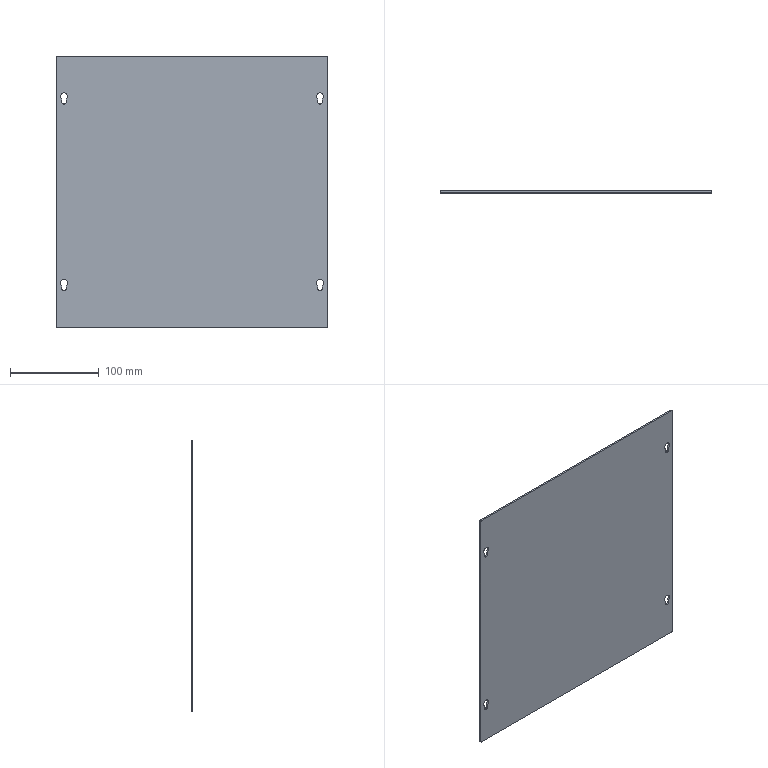Part | SolidWorks | features Fillet 1, FlatPattern 1, ICE 1, LPattern 1, SMBaseFlange 1, SheetMetal 1 | 1 solid | 30 faces | box 304.8 x 2 x 304.8 mm | volume 185210 mm3 | cylinder 16 | plane 14 | commonest cylinder face diameters 8 x8 2 x4 5.4 x4
STEP:
#1=CARTESIAN_POINT('',(-144.,-2.,111.6));
#2=VERTEX_POINT('',#1);
#3=CARTESIAN_POINT('',(-141.3,-2.,104.649));
#4=VERTEX_POINT('',#3);
#5=CARTESIAN_POINT('',(-144.,-2.,107.6));
#6=DIRECTION('',(0.,1.,0.));
#7=DIRECTION('',(0.,0.,1.));
#8=AXIS2_PLACEMENT_3D('',#5,#6,#7);
#9=CIRCLE('',#8,4.);
#10=EDGE_CURVE('',#2,#4,#9,.T.);
#11=ORIENTED_EDGE('',*,*,#10,.F.);
#12=CARTESIAN_POINT('',(-144.,0.,111.6));
#13=VERTEX_POINT('',#12);
#14=CARTESIAN_POINT('',(-144.,-10.,111.6));
#15=DIRECTION('',(0.,1.,0.));
#16=VECTOR('',#15,1000.);
#17=LINE('',#14,#16);
#18=EDGE_CURVE('',#2,#13,#17,.T.);
#19=ORIENTED_EDGE('',*,*,#18,.T.);
#20=CARTESIAN_POINT('',(-141.3,0.,104.649));
#21=VERTEX_POINT('',#20);
#22=CARTESIAN_POINT('',(-144.,0.,107.6));
#23=DIRECTION('',(0.,1.,0.));
#24=DIRECTION('',(0.,0.,1.));
#25=AXIS2_PLACEMENT_3D('',#22,#23,#24);
#26=CIRCLE('',#25,4.);
#27=EDGE_CURVE('',#13,#21,#26,.T.);
#28=ORIENTED_EDGE('',*,*,#27,.T.);
#29=CARTESIAN_POINT('',(-141.3,-10.,104.649));
#30=DIRECTION('',(0.,1.,0.));
#31=VECTOR('',#30,1000.);
#32=LINE('',#29,#31);
#33=EDGE_CURVE('',#4,#21,#32,.T.);
#34=ORIENTED_EDGE('',*,*,#33,.F.);
#35=EDGE_LOOP('',(#11,#19,#28,#34));
#36=FACE_OUTER_BOUND('',#35,.T.);
#37=CARTESIAN_POINT('',(-144.,-10.,107.6));
#38=DIRECTION('',(0.,1.,0.));
#39=DIRECTION('',(0.,0.,1.));
#40=AXIS2_PLACEMENT_3D('',#37,#38,#39);
#41=CYLINDRICAL_SURFACE('',#40,4.);
#42=ADVANCED_FACE('',(#36),#41,.F.);
#43=CARTESIAN_POINT('',(144.,-2.,111.6));
#44=VERTEX_POINT('',#43);
#45=CARTESIAN_POINT('',(146.7,-2.,104.649));
#46=VERTEX_POINT('',#45);
#47=CARTESIAN_POINT('',(144.,-2.,107.6));
#48=DIRECTION('',(0.,1.,0.));
#49=DIRECTION('',(0.,0.,1.));
#50=AXIS2_PLACEMENT_3D('',#47,#48,#49);
#51=CIRCLE('',#50,4.);
#52=EDGE_CURVE('',#44,#46,#51,.T.);
#53=ORIENTED_EDGE('',*,*,#52,.F.);
#54=CARTESIAN_POINT('',(144.,0.,111.6));
#55=VERTEX_POINT('',#54);
#56=CARTESIAN_POINT('',(144.,-10.,111.6));
#57=DIRECTION('',(0.,1.,0.));
#58=VECTOR('',#57,1000.);
#59=LINE('',#56,#58);
#60=EDGE_CURVE('',#44,#55,#59,.T.);
#61=ORIENTED_EDGE('',*,*,#60,.T.);
#62=CARTESIAN_POINT('',(146.7,0.,104.649));
#63=VERTEX_POINT('',#62);
#64=CARTESIAN_POINT('',(144.,0.,107.6));
#65=DIRECTION('',(0.,1.,0.));
#66=DIRECTION('',(0.,0.,-1.));
#67=AXIS2_PLACEMENT_3D('',#64,#65,#66);
#68=CIRCLE('',#67,4.);
#69=EDGE_CURVE('',#55,#63,#68,.T.);
#70=ORIENTED_EDGE('',*,*,#69,.T.);
#71=CARTESIAN_POINT('',(146.7,-10.,104.649));
#72=DIRECTION('',(0.,1.,0.));
#73=VECTOR('',#72,1000.);
#74=LINE('',#71,#73);
#75=EDGE_CURVE('',#46,#63,#74,.T.);
#76=ORIENTED_EDGE('',*,*,#75,.F.);
#77=EDGE_LOOP('',(#53,#61,#70,#76));
#78=FACE_OUTER_BOUND('',#77,.T.);
#79=CARTESIAN_POINT('',(144.,-10.,107.6));
#80=DIRECTION('',(0.,1.,0.));
#81=DIRECTION('',(0.,0.,1.));
#82=AXIS2_PLACEMENT_3D('',#79,#80,#81);
#83=CYLINDRICAL_SURFACE('',#82,4.);
#84=ADVANCED_FACE('',(#78),#83,.F.);
#85=CARTESIAN_POINT('',(-144.,-2.,-98.4));
#86=VERTEX_POINT('',#85);
#87=CARTESIAN_POINT('',(-141.3,-2.,-105.351));
#88=VERTEX_POINT('',#87);
#89=CARTESIAN_POINT('',(-144.,-2.,-102.4));
#90=DIRECTION('',(0.,1.,0.));
#91=DIRECTION('',(0.,0.,1.));
#92=AXIS2_PLACEMENT_3D('',#89,#90,#91);
#93=CIRCLE('',#92,4.);
#94=EDGE_CURVE('',#86,#88,#93,.T.);
#95=ORIENTED_EDGE('',*,*,#94,.F.);
#96=CARTESIAN_POINT('',(-144.,0.,-98.4));
#97=VERTEX_POINT('',#96);
#98=CARTESIAN_POINT('',(-144.,-10.,-98.4));
#99=DIRECTION('',(0.,1.,0.));
#100=VECTOR('',#99,1000.);
#101=LINE('',#98,#100);
#102=EDGE_CURVE('',#86,#97,#101,.T.);
#103=ORIENTED_EDGE('',*,*,#102,.T.);
#104=CARTESIAN_POINT('',(-141.3,0.,-105.351));
#105=VERTEX_POINT('',#104);
#106=CARTESIAN_POINT('',(-144.,0.,-102.4));
#107=DIRECTION('',(0.,1.,0.));
#108=DIRECTION('',(0.,0.,1.));
#109=AXIS2_PLACEMENT_3D('',#106,#107,#108);
#110=CIRCLE('',#109,4.);
#111=EDGE_CURVE('',#97,#105,#110,.T.);
#112=ORIENTED_EDGE('',*,*,#111,.T.);
#113=CARTESIAN_POINT('',(-141.3,-10.,-105.351));
#114=DIRECTION('',(0.,1.,0.));
#115=VECTOR('',#114,1000.);
#116=LINE('',#113,#115);
#117=EDGE_CURVE('',#88,#105,#116,.T.);
#118=ORIENTED_EDGE('',*,*,#117,.F.);
#119=EDGE_LOOP('',(#95,#103,#112,#118));
#120=FACE_OUTER_BOUND('',#119,.T.);
#121=CARTESIAN_POINT('',(-144.,-10.,-102.4));
#122=DIRECTION('',(0.,1.,0.));
#123=DIRECTION('',(0.,0.,1.));
#124=AXIS2_PLACEMENT_3D('',#121,#122,#123);
#125=CYLINDRICAL_SURFACE('',#124,4.);
#126=ADVANCED_FACE('',(#120),#125,.F.);
#127=CARTESIAN_POINT('',(144.,-2.,-98.4));
#128=VERTEX_POINT('',#127);
#129=CARTESIAN_POINT('',(146.7,-2.,-105.351));
#130=VERTEX_POINT('',#129);
#131=CARTESIAN_POINT('',(144.,-2.,-102.4));
#132=DIRECTION('',(0.,1.,0.));
#133=DIRECTION('',(0.,0.,1.));
#134=AXIS2_PLACEMENT_3D('',#131,#132,#133);
#135=CIRCLE('',#134,4.);
#136=EDGE_CURVE('',#128,#130,#135,.T.);
#137=ORIENTED_EDGE('',*,*,#136,.F.);
#138=CARTESIAN_POINT('',(144.,0.,-98.4));
#139=VERTEX_POINT('',#138);
#140=CARTESIAN_POINT('',(144.,-10.,-98.4));
#141=DIRECTION('',(0.,1.,0.));
#142=VECTOR('',#141,1000.);
#143=LINE('',#140,#142);
#144=EDGE_CURVE('',#128,#139,#143,.T.);
#145=ORIENTED_EDGE('',*,*,#144,.T.);
#146=CARTESIAN_POINT('',(146.7,0.,-105.351));
#147=VERTEX_POINT('',#146);
#148=CARTESIAN_POINT('',(144.,0.,-102.4));
#149=DIRECTION('',(0.,1.,0.));
#150=DIRECTION('',(0.,0.,-1.));
#151=AXIS2_PLACEMENT_3D('',#148,#149,#150);
#152=CIRCLE('',#151,4.);
#153=EDGE_CURVE('',#139,#147,#152,.T.);
#154=ORIENTED_EDGE('',*,*,#153,.T.);
#155=CARTESIAN_POINT('',(146.7,-10.,-105.351));
#156=DIRECTION('',(0.,1.,0.));
#157=VECTOR('',#156,1000.);
#158=LINE('',#155,#157);
#159=EDGE_CURVE('',#130,#147,#158,.T.);
#160=ORIENTED_EDGE('',*,*,#159,.F.);
#161=EDGE_LOOP('',(#137,#145,#154,#160));
#162=FACE_OUTER_BOUND('',#161,.T.);
#163=CARTESIAN_POINT('',(144.,-10.,-102.4));
#164=DIRECTION('',(0.,1.,0.));
#165=DIRECTION('',(0.,0.,1.));
#166=AXIS2_PLACEMENT_3D('',#163,#164,#165);
#167=CYLINDRICAL_SURFACE('',#166,4.);
#168=ADVANCED_FACE('',(#162),#167,.F.);
#169=CARTESIAN_POINT('',(152.4,-2.,151.4));
#170=VERTEX_POINT('',#169);
#171=CARTESIAN_POINT('',(152.4,-2.,-151.4));
#172=VERTEX_POINT('',#171);
#173=CARTESIAN_POINT('',(152.4,-2.,-152.4));
#174=DIRECTION('',(0.,0.,-1.));
#175=VECTOR('',#174,1000.);
#176=LINE('',#173,#175);
#177=EDGE_CURVE('',#170,#172,#176,.T.);
#178=ORIENTED_EDGE('',*,*,#177,.T.);
#179=CARTESIAN_POINT('',(152.4,0.,-151.4));
#180=VERTEX_POINT('',#179);
#181=CARTESIAN_POINT('',(152.4,-2.,-151.4));
#182=DIRECTION('',(0.,1.,0.));
#183=VECTOR('',#182,1000.);
#184=LINE('',#181,#183);
#185=EDGE_CURVE('',#172,#180,#184,.T.);
#186=ORIENTED_EDGE('',*,*,#185,.T.);
#187=CARTESIAN_POINT('',(152.4,0.,151.4));
#188=VERTEX_POINT('',#187);
#189=CARTESIAN_POINT('',(152.4,0.,-152.4));
#190=DIRECTION('',(0.,0.,-1.));
#191=VECTOR('',#190,1000.);
#192=LINE('',#189,#191);
#193=EDGE_CURVE('',#188,#180,#192,.T.);
#194=ORIENTED_EDGE('',*,*,#193,.F.);
#195=CARTESIAN_POINT('',(152.4,-2.,151.4));
#196=DIRECTION('',(0.,-1.,0.));
#197=VECTOR('',#196,1000.);
#198=LINE('',#195,#197);
#199=EDGE_CURVE('',#188,#170,#198,.T.);
#200=ORIENTED_EDGE('',*,*,#199,.T.);
#201=EDGE_LOOP('',(#178,#186,#194,#200));
#202=FACE_OUTER_BOUND('',#201,.T.);
#203=CARTESIAN_POINT('',(152.4,-2.,-152.4));
#204=DIRECTION('',(1.,0.,0.));
#205=DIRECTION('',(0.,0.,-1.));
#206=AXIS2_PLACEMENT_3D('',#203,#204,#205);
#207=PLANE('',#206);
#208=ADVANCED_FACE('',(#202),#207,.T.);
#209=CARTESIAN_POINT('',(-151.4,-2.,152.4));
#210=VERTEX_POINT('',#209);
#211=CARTESIAN_POINT('',(151.4,-2.,152.4));
#212=VERTEX_POINT('',#211);
#213=CARTESIAN_POINT('',(-152.4,-2.,152.4));
#214=DIRECTION('',(1.,0.,0.));
#215=VECTOR('',#214,1000.);
#216=LINE('',#213,#215);
#217=EDGE_CURVE('',#210,#212,#216,.T.);
#218=ORIENTED_EDGE('',*,*,#217,.T.);
#219=CARTESIAN_POINT('',(151.4,0.,152.4));
#220=VERTEX_POINT('',#219);
#221=CARTESIAN_POINT('',(151.4,-2.,152.4));
#222=DIRECTION('',(0.,1.,0.));
#223=VECTOR('',#222,1000.);
#224=LINE('',#221,#223);
#225=EDGE_CURVE('',#212,#220,#224,.T.);
#226=ORIENTED_EDGE('',*,*,#225,.T.);
#227=CARTESIAN_POINT('',(-151.4,0.,152.4));
#228=VERTEX_POINT('',#227);
#229=CARTESIAN_POINT('',(-152.4,0.,152.4));
#230=DIRECTION('',(1.,0.,0.));
#231=VECTOR('',#230,1000.);
#232=LINE('',#229,#231);
#233=EDGE_CURVE('',#228,#220,#232,.T.);
#234=ORIENTED_EDGE('',*,*,#233,.F.);
#235=CARTESIAN_POINT('',(-151.4,-2.,152.4));
#236=DIRECTION('',(0.,-1.,0.));
#237=VECTOR('',#236,1000.);
#238=LINE('',#235,#237);
#239=EDGE_CURVE('',#228,#210,#238,.T.);
#240=ORIENTED_EDGE('',*,*,#239,.T.);
#241=EDGE_LOOP('',(#218,#226,#234,#240));
#242=FACE_OUTER_BOUND('',#241,.T.);
#243=CARTESIAN_POINT('',(-152.4,-2.,152.4));
#244=DIRECTION('',(0.,0.,1.));
#245=DIRECTION('',(1.,0.,0.));
#246=AXIS2_PLACEMENT_3D('',#243,#244,#245);
#247=PLANE('',#246);
#248=ADVANCED_FACE('',(#242),#247,.T.);
#249=CARTESIAN_POINT('',(-152.4,0.,-151.4));
#250=VERTEX_POINT('',#249);
#251=CARTESIAN_POINT('',(-152.4,0.,151.4));
#252=VERTEX_POINT('',#251);
#253=CARTESIAN_POINT('',(-152.4,0.,-152.4));
#254=DIRECTION('',(0.,0.,1.));
#255=VECTOR('',#254,1000.);
#256=LINE('',#253,#255);
#257=EDGE_CURVE('',#250,#252,#256,.T.);
#258=ORIENTED_EDGE('',*,*,#257,.F.);
#259=CARTESIAN_POINT('',(-152.4,-2.,-151.4));
#260=VERTEX_POINT('',#259);
#261=CARTESIAN_POINT('',(-152.4,-2.,-151.4));
#262=DIRECTION('',(0.,-1.,0.));
#263=VECTOR('',#262,1000.);
#264=LINE('',#261,#263);
#265=EDGE_CURVE('',#250,#260,#264,.T.);
#266=ORIENTED_EDGE('',*,*,#265,.T.);
#267=CARTESIAN_POINT('',(-152.4,-2.,151.4));
#268=VERTEX_POINT('',#267);
#269=CARTESIAN_POINT('',(-152.4,-2.,-152.4));
#270=DIRECTION('',(0.,0.,1.));
#271=VECTOR('',#270,1000.);
#272=LINE('',#269,#271);
#273=EDGE_CURVE('',#260,#268,#272,.T.);
#274=ORIENTED_EDGE('',*,*,#273,.T.);
#275=CARTESIAN_POINT('',(-152.4,-2.,151.4));
#276=DIRECTION('',(0.,1.,0.));
#277=VECTOR('',#276,1000.);
#278=LINE('',#275,#277);
#279=EDGE_CURVE('',#268,#252,#278,.T.);
#280=ORIENTED_EDGE('',*,*,#279,.T.);
#281=EDGE_LOOP('',(#258,#266,#274,#280));
#282=FACE_OUTER_BOUND('',#281,.T.);
#283=CARTESIAN_POINT('',(-152.4,-2.,-152.4));
#284=DIRECTION('',(-1.,0.,0.));
#285=DIRECTION('',(0.,0.,1.));
#286=AXIS2_PLACEMENT_3D('',#283,#284,#285);
#287=PLANE('',#286);
#288=ADVANCED_FACE('',(#282),#287,.T.);
#289=CARTESIAN_POINT('',(151.4,-2.,-152.4));
#290=VERTEX_POINT('',#289);
#291=CARTESIAN_POINT('',(-151.4,-2.,-152.4));
#292=VERTEX_POINT('',#291);
#293=CARTESIAN_POINT('',(-152.4,-2.,-152.4));
#294=DIRECTION('',(-1.,0.,0.));
#295=VECTOR('',#294,1000.);
#296=LINE('',#293,#295);
#297=EDGE_CURVE('',#290,#292,#296,.T.);
#298=ORIENTED_EDGE('',*,*,#297,.T.);
#299=CARTESIAN_POINT('',(-151.4,0.,-152.4));
#300=VERTEX_POINT('',#299);
#301=CARTESIAN_POINT('',(-151.4,-2.,-152.4));
#302=DIRECTION('',(0.,1.,0.));
#303=VECTOR('',#302,1000.);
#304=LINE('',#301,#303);
#305=EDGE_CURVE('',#292,#300,#304,.T.);
#306=ORIENTED_EDGE('',*,*,#305,.T.);
#307=CARTESIAN_POINT('',(151.4,0.,-152.4));
#308=VERTEX_POINT('',#307);
#309=CARTESIAN_POINT('',(-152.4,0.,-152.4));
#310=DIRECTION('',(-1.,0.,0.));
#311=VECTOR('',#310,1000.);
#312=LINE('',#309,#311);
#313=EDGE_CURVE('',#308,#300,#312,.T.);
#314=ORIENTED_EDGE('',*,*,#313,.F.);
#315=CARTESIAN_POINT('',(151.4,-2.,-152.4));
#316=DIRECTION('',(0.,-1.,0.));
#317=VECTOR('',#316,1000.);
#318=LINE('',#315,#317);
#319=EDGE_CURVE('',#308,#290,#318,.T.);
#320=ORIENTED_EDGE('',*,*,#319,.T.);
#321=EDGE_LOOP('',(#298,#306,#314,#320));
#322=FACE_OUTER_BOUND('',#321,.T.);
#323=CARTESIAN_POINT('',(-152.4,-2.,-152.4));
#324=DIRECTION('',(0.,0.,-1.));
#325=DIRECTION('',(-1.,0.,0.));
#326=AXIS2_PLACEMENT_3D('',#323,#324,#325);
#327=PLANE('',#326);
#328=ADVANCED_FACE('',(#322),#327,.T.);
#329=CARTESIAN_POINT('',(-146.7,-2.,101.6));
#330=VERTEX_POINT('',#329);
#331=CARTESIAN_POINT('',(-146.7,-2.,104.649));
#332=VERTEX_POINT('',#331);
#333=CARTESIAN_POINT('',(-146.7,-2.,0.));
#334=DIRECTION('',(0.,0.,1.));
#335=VECTOR('',#334,1000.);
#336=LINE('',#333,#335);
#337=EDGE_CURVE('',#330,#332,#336,.T.);
#338=ORIENTED_EDGE('',*,*,#337,.T.);
#339=CARTESIAN_POINT('',(-144.,-2.,107.6));
#340=DIRECTION('',(0.,1.,0.));
#341=DIRECTION('',(0.,0.,1.));
#342=AXIS2_PLACEMENT_3D('',#339,#340,#341);
#343=CIRCLE('',#342,4.);
#344=EDGE_CURVE('',#332,#2,#343,.T.);
#345=ORIENTED_EDGE('',*,*,#344,.T.);
#346=ORIENTED_EDGE('',*,*,#10,.T.);
#347=CARTESIAN_POINT('',(-141.3,-2.,101.6));
#348=VERTEX_POINT('',#347);
#349=CARTESIAN_POINT('',(-141.3,-2.,0.));
#350=DIRECTION('',(0.,0.,-1.));
#351=VECTOR('',#350,1000.);
#352=LINE('',#349,#351);
#353=EDGE_CURVE('',#4,#348,#352,.T.);
#354=ORIENTED_EDGE('',*,*,#353,.T.);
#355=CARTESIAN_POINT('',(-144.,-2.,101.6));
#356=DIRECTION('',(0.,1.,0.));
#357=DIRECTION('',(0.,0.,1.));
#358=AXIS2_PLACEMENT_3D('',#355,#356,#357);
#359=CIRCLE('',#358,2.7);
#360=EDGE_CURVE('',#348,#330,#359,.T.);
#361=ORIENTED_EDGE('',*,*,#360,.T.);
#362=EDGE_LOOP('',(#338,#345,#346,#354,#361));
#363=FACE_BOUND('',#362,.T.);
#364=CARTESIAN_POINT('',(146.7,-2.,101.6));
#365=VERTEX_POINT('',#364);
#366=CARTESIAN_POINT('',(146.7,-2.,0.));
#367=DIRECTION('',(0.,0.,-1.));
#368=VECTOR('',#367,1000.);
#369=LINE('',#366,#368);
#370=EDGE_CURVE('',#46,#365,#369,.T.);
#371=ORIENTED_EDGE('',*,*,#370,.T.);
#372=CARTESIAN_POINT('',(141.3,-2.,101.6));
#373=VERTEX_POINT('',#372);
#374=CARTESIAN_POINT('',(144.,-2.,101.6));
#375=DIRECTION('',(0.,1.,0.));
#376=DIRECTION('',(0.,0.,1.));
#377=AXIS2_PLACEMENT_3D('',#374,#375,#376);
#378=CIRCLE('',#377,2.7);
#379=EDGE_CURVE('',#365,#373,#378,.T.);
#380=ORIENTED_EDGE('',*,*,#379,.T.);
#381=CARTESIAN_POINT('',(141.3,-2.,104.649));
#382=VERTEX_POINT('',#381);
#383=CARTESIAN_POINT('',(141.3,-2.,0.));
#384=DIRECTION('',(0.,0.,1.));
#385=VECTOR('',#384,1000.);
#386=LINE('',#383,#385);
#387=EDGE_CURVE('',#373,#382,#386,.T.);
#388=ORIENTED_EDGE('',*,*,#387,.T.);
#389=CARTESIAN_POINT('',(144.,-2.,107.6));
#390=DIRECTION('',(0.,1.,0.));
#391=DIRECTION('',(0.,0.,1.));
#392=AXIS2_PLACEMENT_3D('',#389,#390,#391);
#393=CIRCLE('',#392,4.);
#394=EDGE_CURVE('',#382,#44,#393,.T.);
#395=ORIENTED_EDGE('',*,*,#394,.T.);
#396=ORIENTED_EDGE('',*,*,#52,.T.);
#397=EDGE_LOOP('',(#371,#380,#388,#395,#396));
#398=FACE_BOUND('',#397,.T.);
#399=CARTESIAN_POINT('',(-146.7,-2.,-108.4));
#400=VERTEX_POINT('',#399);
#401=CARTESIAN_POINT('',(-146.7,-2.,-105.351));
#402=VERTEX_POINT('',#401);
#403=CARTESIAN_POINT('',(-146.7,-2.,0.));
#404=DIRECTION('',(0.,0.,1.));
#405=VECTOR('',#404,1000.);
#406=LINE('',#403,#405);
#407=EDGE_CURVE('',#400,#402,#406,.T.);
#408=ORIENTED_EDGE('',*,*,#407,.T.);
#409=CARTESIAN_POINT('',(-144.,-2.,-102.4));
#410=DIRECTION('',(0.,1.,0.));
#411=DIRECTION('',(0.,0.,1.));
#412=AXIS2_PLACEMENT_3D('',#409,#410,#411);
#413=CIRCLE('',#412,4.);
#414=EDGE_CURVE('',#402,#86,#413,.T.);
#415=ORIENTED_EDGE('',*,*,#414,.T.);
#416=ORIENTED_EDGE('',*,*,#94,.T.);
#417=CARTESIAN_POINT('',(-141.3,-2.,-108.4));
#418=VERTEX_POINT('',#417);
#419=CARTESIAN_POINT('',(-141.3,-2.,0.));
#420=DIRECTION('',(0.,0.,-1.));
#421=VECTOR('',#420,1000.);
#422=LINE('',#419,#421);
#423=EDGE_CURVE('',#88,#418,#422,.T.);
#424=ORIENTED_EDGE('',*,*,#423,.T.);
#425=CARTESIAN_POINT('',(-144.,-2.,-108.4));
#426=DIRECTION('',(0.,1.,0.));
#427=DIRECTION('',(0.,0.,1.));
#428=AXIS2_PLACEMENT_3D('',#425,#426,#427);
#429=CIRCLE('',#428,2.7);
#430=EDGE_CURVE('',#418,#400,#429,.T.);
#431=ORIENTED_EDGE('',*,*,#430,.T.);
#432=EDGE_LOOP('',(#408,#415,#416,#424,#431));
#433=FACE_BOUND('',#432,.T.);
#434=CARTESIAN_POINT('',(146.7,-2.,-108.4));
#435=VERTEX_POINT('',#434);
#436=CARTESIAN_POINT('',(146.7,-2.,0.));
#437=DIRECTION('',(0.,0.,-1.));
#438=VECTOR('',#437,1000.);
#439=LINE('',#436,#438);
#440=EDGE_CURVE('',#130,#435,#439,.T.);
#441=ORIENTED_EDGE('',*,*,#440,.T.);
#442=CARTESIAN_POINT('',(141.3,-2.,-108.4));
#443=VERTEX_POINT('',#442);
#444=CARTESIAN_POINT('',(144.,-2.,-108.4));
#445=DIRECTION('',(0.,1.,0.));
#446=DIRECTION('',(0.,0.,1.));
#447=AXIS2_PLACEMENT_3D('',#444,#445,#446);
#448=CIRCLE('',#447,2.7);
#449=EDGE_CURVE('',#435,#443,#448,.T.);
#450=ORIENTED_EDGE('',*,*,#449,.T.);
#451=CARTESIAN_POINT('',(141.3,-2.,-105.351));
#452=VERTEX_POINT('',#451);
#453=CARTESIAN_POINT('',(141.3,-2.,0.));
#454=DIRECTION('',(0.,0.,1.));
#455=VECTOR('',#454,1000.);
#456=LINE('',#453,#455);
#457=EDGE_CURVE('',#443,#452,#456,.T.);
#458=ORIENTED_EDGE('',*,*,#457,.T.);
#459=CARTESIAN_POINT('',(144.,-2.,-102.4));
#460=DIRECTION('',(0.,1.,0.));
#461=DIRECTION('',(0.,0.,1.));
#462=AXIS2_PLACEMENT_3D('',#459,#460,#461);
#463=CIRCLE('',#462,4.);
#464=EDGE_CURVE('',#452,#128,#463,.T.);
#465=ORIENTED_EDGE('',*,*,#464,.T.);
#466=ORIENTED_EDGE('',*,*,#136,.T.);
#467=EDGE_LOOP('',(#441,#450,#458,#465,#466));
#468=FACE_BOUND('',#467,.T.);
#469=ORIENTED_EDGE('',*,*,#273,.F.);
#470=CARTESIAN_POINT('',(-151.4,-2.,-151.4));
#471=DIRECTION('',(0.,-1.,0.));
#472=DIRECTION('',(0.,0.,1.));
#473=AXIS2_PLACEMENT_3D('',#470,#471,#472);
#474=CIRCLE('',#473,1.);
#475=EDGE_CURVE('',#260,#292,#474,.T.);
#476=ORIENTED_EDGE('',*,*,#475,.T.);
#477=ORIENTED_EDGE('',*,*,#297,.F.);
#478=CARTESIAN_POINT('',(151.4,-2.,-151.4));
#479=DIRECTION('',(0.,-1.,0.));
#480=DIRECTION('',(0.,0.,1.));
#481=AXIS2_PLACEMENT_3D('',#478,#479,#480);
#482=CIRCLE('',#481,1.);
#483=EDGE_CURVE('',#290,#172,#482,.T.);
#484=ORIENTED_EDGE('',*,*,#483,.T.);
#485=ORIENTED_EDGE('',*,*,#177,.F.);
#486=CARTESIAN_POINT('',(151.4,-2.,151.4));
#487=DIRECTION('',(0.,-1.,0.));
#488=DIRECTION('',(0.,0.,1.));
#489=AXIS2_PLACEMENT_3D('',#486,#487,#488);
#490=CIRCLE('',#489,1.);
#491=EDGE_CURVE('',#170,#212,#490,.T.);
#492=ORIENTED_EDGE('',*,*,#491,.T.);
#493=ORIENTED_EDGE('',*,*,#217,.F.);
#494=CARTESIAN_POINT('',(-151.4,-2.,151.4));
#495=DIRECTION('',(0.,-1.,0.));
#496=DIRECTION('',(0.,0.,1.));
#497=AXIS2_PLACEMENT_3D('',#494,#495,#496);
#498=CIRCLE('',#497,1.);
#499=EDGE_CURVE('',#210,#268,#498,.T.);
#500=ORIENTED_EDGE('',*,*,#499,.T.);
#501=EDGE_LOOP('',(#469,#476,#477,#484,#485,#492,#493,#500));
#502=FACE_OUTER_BOUND('',#501,.T.);
#503=CARTESIAN_POINT('',(0.,-2.,0.));
#504=DIRECTION('',(0.,1.,0.));
#505=DIRECTION('',(0.,0.,1.));
#506=AXIS2_PLACEMENT_3D('',#503,#504,#505);
#507=PLANE('',#506);
#508=ADVANCED_FACE('',(#363,#398,#433,#468,#502),#507,.F.);
#509=CARTESIAN_POINT('',(-146.7,0.,104.649));
#510=VERTEX_POINT('',#509);
#511=CARTESIAN_POINT('',(-144.,0.,107.6));
#512=DIRECTION('',(0.,1.,0.));
#513=DIRECTION('',(0.,0.,1.));
#514=AXIS2_PLACEMENT_3D('',#511,#512,#513);
#515=CIRCLE('',#514,4.);
#516=EDGE_CURVE('',#510,#13,#515,.T.);
#517=ORIENTED_EDGE('',*,*,#516,.F.);
#518=CARTESIAN_POINT('',(-146.7,0.,101.6));
#519=VERTEX_POINT('',#518);
#520=CARTESIAN_POINT('',(-146.7,0.,101.6));
#521=DIRECTION('',(0.,0.,1.));
#522=VECTOR('',#521,1000.);
#523=LINE('',#520,#522);
#524=EDGE_CURVE('',#519,#510,#523,.T.);
#525=ORIENTED_EDGE('',*,*,#524,.F.);
#526=CARTESIAN_POINT('',(-141.3,0.,101.6));
#527=VERTEX_POINT('',#526);
#528=CARTESIAN_POINT('',(-144.,0.,101.6));
#529=DIRECTION('',(0.,1.,0.));
#530=DIRECTION('',(0.,0.,1.));
#531=AXIS2_PLACEMENT_3D('',#528,#529,#530);
#532=CIRCLE('',#531,2.7);
#533=EDGE_CURVE('',#527,#519,#532,.T.);
#534=ORIENTED_EDGE('',*,*,#533,.F.);
#535=CARTESIAN_POINT('',(-141.3,0.,101.6));
#536=DIRECTION('',(0.,0.,-1.));
#537=VECTOR('',#536,1000.);
#538=LINE('',#535,#537);
#539=EDGE_CURVE('',#21,#527,#538,.T.);
#540=ORIENTED_EDGE('',*,*,#539,.F.);
#541=ORIENTED_EDGE('',*,*,#27,.F.);
#542=EDGE_LOOP('',(#517,#525,#534,#540,#541));
#543=FACE_BOUND('',#542,.T.);
#544=CARTESIAN_POINT('',(146.7,0.,101.6));
#545=VERTEX_POINT('',#544);
#546=CARTESIAN_POINT('',(141.3,0.,101.6));
#547=VERTEX_POINT('',#546);
#548=CARTESIAN_POINT('',(144.,0.,101.6));
#549=DIRECTION('',(0.,1.,0.));
#550=DIRECTION('',(0.,0.,-1.));
#551=AXIS2_PLACEMENT_3D('',#548,#549,#550);
#552=CIRCLE('',#551,2.7);
#553=EDGE_CURVE('',#545,#547,#552,.T.);
#554=ORIENTED_EDGE('',*,*,#553,.F.);
#555=CARTESIAN_POINT('',(146.7,0.,101.6));
#556=DIRECTION('',(0.,0.,-1.));
#557=VECTOR('',#556,1000.);
#558=LINE('',#555,#557);
#559=EDGE_CURVE('',#63,#545,#558,.T.);
#560=ORIENTED_EDGE('',*,*,#559,.F.);
#561=ORIENTED_EDGE('',*,*,#69,.F.);
#562=CARTESIAN_POINT('',(141.3,0.,104.649));
#563=VERTEX_POINT('',#562);
#564=CARTESIAN_POINT('',(144.,0.,107.6));
#565=DIRECTION('',(0.,1.,0.));
#566=DIRECTION('',(0.,0.,-1.));
#567=AXIS2_PLACEMENT_3D('',#564,#565,#566);
#568=CIRCLE('',#567,4.);
#569=EDGE_CURVE('',#563,#55,#568,.T.);
#570=ORIENTED_EDGE('',*,*,#569,.F.);
#571=CARTESIAN_POINT('',(141.3,0.,101.6));
#572=DIRECTION('',(0.,0.,1.));
#573=VECTOR('',#572,1000.);
#574=LINE('',#571,#573);
#575=EDGE_CURVE('',#547,#563,#574,.T.);
#576=ORIENTED_EDGE('',*,*,#575,.F.);
#577=EDGE_LOOP('',(#554,#560,#561,#570,#576));
#578=FACE_BOUND('',#577,.T.);
#579=CARTESIAN_POINT('',(-146.7,0.,-105.351));
#580=VERTEX_POINT('',#579);
#581=CARTESIAN_POINT('',(-144.,0.,-102.4));
#582=DIRECTION('',(0.,1.,0.));
#583=DIRECTION('',(0.,0.,1.));
#584=AXIS2_PLACEMENT_3D('',#581,#582,#583);
#585=CIRCLE('',#584,4.);
#586=EDGE_CURVE('',#580,#97,#585,.T.);
#587=ORIENTED_EDGE('',*,*,#586,.F.);
#588=CARTESIAN_POINT('',(-146.7,0.,-108.4));
#589=VERTEX_POINT('',#588);
#590=CARTESIAN_POINT('',(-146.7,0.,-108.4));
#591=DIRECTION('',(0.,0.,1.));
#592=VECTOR('',#591,1000.);
#593=LINE('',#590,#592);
#594=EDGE_CURVE('',#589,#580,#593,.T.);
#595=ORIENTED_EDGE('',*,*,#594,.F.);
#596=CARTESIAN_POINT('',(-141.3,0.,-108.4));
#597=VERTEX_POINT('',#596);
#598=CARTESIAN_POINT('',(-144.,0.,-108.4));
#599=DIRECTION('',(0.,1.,0.));
#600=DIRECTION('',(0.,0.,1.));
#601=AXIS2_PLACEMENT_3D('',#598,#599,#600);
#602=CIRCLE('',#601,2.7);
#603=EDGE_CURVE('',#597,#589,#602,.T.);
#604=ORIENTED_EDGE('',*,*,#603,.F.);
#605=CARTESIAN_POINT('',(-141.3,0.,-108.4));
#606=DIRECTION('',(0.,0.,-1.));
#607=VECTOR('',#606,1000.);
#608=LINE('',#605,#607);
#609=EDGE_CURVE('',#105,#597,#608,.T.);
#610=ORIENTED_EDGE('',*,*,#609,.F.);
#611=ORIENTED_EDGE('',*,*,#111,.F.);
#612=EDGE_LOOP('',(#587,#595,#604,#610,#611));
#613=FACE_BOUND('',#612,.T.);
#614=CARTESIAN_POINT('',(146.7,0.,-108.4));
#615=VERTEX_POINT('',#614);
#616=CARTESIAN_POINT('',(141.3,0.,-108.4));
#617=VERTEX_POINT('',#616);
#618=CARTESIAN_POINT('',(144.,0.,-108.4));
#619=DIRECTION('',(0.,1.,0.));
#620=DIRECTION('',(0.,0.,-1.));
#621=AXIS2_PLACEMENT_3D('',#618,#619,#620);
#622=CIRCLE('',#621,2.7);
#623=EDGE_CURVE('',#615,#617,#622,.T.);
#624=ORIENTED_EDGE('',*,*,#623,.F.);
#625=CARTESIAN_POINT('',(146.7,0.,-108.4));
#626=DIRECTION('',(0.,0.,-1.));
#627=VECTOR('',#626,1000.);
#628=LINE('',#625,#627);
#629=EDGE_CURVE('',#147,#615,#628,.T.);
#630=ORIENTED_EDGE('',*,*,#629,.F.);
#631=ORIENTED_EDGE('',*,*,#153,.F.);
#632=CARTESIAN_POINT('',(141.3,0.,-105.351));
#633=VERTEX_POINT('',#632);
#634=CARTESIAN_POINT('',(144.,0.,-102.4));
#635=DIRECTION('',(0.,1.,0.));
#636=DIRECTION('',(0.,0.,-1.));
#637=AXIS2_PLACEMENT_3D('',#634,#635,#636);
#638=CIRCLE('',#637,4.);
#639=EDGE_CURVE('',#633,#139,#638,.T.);
#640=ORIENTED_EDGE('',*,*,#639,.F.);
#641=CARTESIAN_POINT('',(141.3,0.,-108.4));
#642=DIRECTION('',(0.,0.,1.));
#643=VECTOR('',#642,1000.);
#644=LINE('',#641,#643);
#645=EDGE_CURVE('',#617,#633,#644,.T.);
#646=ORIENTED_EDGE('',*,*,#645,.F.);
#647=EDGE_LOOP('',(#624,#630,#631,#640,#646));
#648=FACE_BOUND('',#647,.T.);
#649=ORIENTED_EDGE('',*,*,#313,.T.);
#650=CARTESIAN_POINT('',(-151.4,0.,-151.4));
#651=DIRECTION('',(0.,1.,0.));
#652=DIRECTION('',(0.,0.,1.));
#653=AXIS2_PLACEMENT_3D('',#650,#651,#652);
#654=CIRCLE('',#653,1.);
#655=EDGE_CURVE('',#300,#250,#654,.T.);
#656=ORIENTED_EDGE('',*,*,#655,.T.);
#657=ORIENTED_EDGE('',*,*,#257,.T.);
#658=CARTESIAN_POINT('',(-151.4,0.,151.4));
#659=DIRECTION('',(0.,1.,0.));
#660=DIRECTION('',(0.,0.,1.));
#661=AXIS2_PLACEMENT_3D('',#658,#659,#660);
#662=CIRCLE('',#661,1.);
#663=EDGE_CURVE('',#252,#228,#662,.T.);
#664=ORIENTED_EDGE('',*,*,#663,.T.);
#665=ORIENTED_EDGE('',*,*,#233,.T.);
#666=CARTESIAN_POINT('',(151.4,0.,151.4));
#667=DIRECTION('',(0.,1.,0.));
#668=DIRECTION('',(0.,0.,1.));
#669=AXIS2_PLACEMENT_3D('',#666,#667,#668);
#670=CIRCLE('',#669,1.);
#671=EDGE_CURVE('',#220,#188,#670,.T.);
#672=ORIENTED_EDGE('',*,*,#671,.T.);
#673=ORIENTED_EDGE('',*,*,#193,.T.);
#674=CARTESIAN_POINT('',(151.4,0.,-151.4));
#675=DIRECTION('',(0.,1.,0.));
#676=DIRECTION('',(0.,0.,1.));
#677=AXIS2_PLACEMENT_3D('',#674,#675,#676);
#678=CIRCLE('',#677,1.);
#679=EDGE_CURVE('',#180,#308,#678,.T.);
#680=ORIENTED_EDGE('',*,*,#679,.T.);
#681=EDGE_LOOP('',(#649,#656,#657,#664,#665,#672,#673,#680));
#682=FACE_OUTER_BOUND('',#681,.T.);
#683=CARTESIAN_POINT('',(0.,0.,0.));
#684=DIRECTION('',(0.,1.,0.));
#685=DIRECTION('',(0.,0.,1.));
#686=AXIS2_PLACEMENT_3D('',#683,#684,#685);
#687=PLANE('',#686);
#688=ADVANCED_FACE('',(#543,#578,#613,#648,#682),#687,.T.);
#689=CARTESIAN_POINT('',(146.7,-10.,-108.4));
#690=DIRECTION('',(0.,1.,0.));
#691=VECTOR('',#690,1000.);
#692=LINE('',#689,#691);
#693=EDGE_CURVE('',#435,#615,#692,.T.);
#694=ORIENTED_EDGE('',*,*,#693,.T.);
#695=ORIENTED_EDGE('',*,*,#623,.T.);
#696=CARTESIAN_POINT('',(141.3,-10.,-108.4));
#697=DIRECTION('',(0.,1.,0.));
#698=VECTOR('',#697,1000.);
#699=LINE('',#696,#698);
#700=EDGE_CURVE('',#443,#617,#699,.T.);
#701=ORIENTED_EDGE('',*,*,#700,.F.);
#702=ORIENTED_EDGE('',*,*,#449,.F.);
#703=EDGE_LOOP('',(#694,#695,#701,#702));
#704=FACE_OUTER_BOUND('',#703,.T.);
#705=CARTESIAN_POINT('',(144.,-10.,-108.4));
#706=DIRECTION('',(0.,1.,0.));
#707=DIRECTION('',(0.,0.,1.));
#708=AXIS2_PLACEMENT_3D('',#705,#706,#707);
#709=CYLINDRICAL_SURFACE('',#708,2.7);
#710=ADVANCED_FACE('',(#704),#709,.F.);
#711=ORIENTED_EDGE('',*,*,#159,.T.);
#712=ORIENTED_EDGE('',*,*,#629,.T.);
#713=ORIENTED_EDGE('',*,*,#693,.F.);
#714=ORIENTED_EDGE('',*,*,#440,.F.);
#715=EDGE_LOOP('',(#711,#712,#713,#714));
#716=FACE_OUTER_BOUND('',#715,.T.);
#717=CARTESIAN_POINT('',(146.7,-10.,-108.4));
#718=DIRECTION('',(1.,0.,0.));
#719=DIRECTION('',(0.,0.,-1.));
#720=AXIS2_PLACEMENT_3D('',#717,#718,#719);
#721=PLANE('',#720);
#722=ADVANCED_FACE('',(#716),#721,.F.);
#723=ORIENTED_EDGE('',*,*,#144,.F.);
#724=ORIENTED_EDGE('',*,*,#464,.F.);
#725=CARTESIAN_POINT('',(141.3,-10.,-105.351));
#726=DIRECTION('',(0.,1.,0.));
#727=VECTOR('',#726,1000.);
#728=LINE('',#725,#727);
#729=EDGE_CURVE('',#452,#633,#728,.T.);
#730=ORIENTED_EDGE('',*,*,#729,.T.);
#731=ORIENTED_EDGE('',*,*,#639,.T.);
#732=EDGE_LOOP('',(#723,#724,#730,#731));
#733=FACE_OUTER_BOUND('',#732,.T.);
#734=CARTESIAN_POINT('',(144.,-10.,-102.4));
#735=DIRECTION('',(0.,1.,0.));
#736=DIRECTION('',(0.,0.,1.));
#737=AXIS2_PLACEMENT_3D('',#734,#735,#736);
#738=CYLINDRICAL_SURFACE('',#737,4.);
#739=ADVANCED_FACE('',(#733),#738,.F.);
#740=ORIENTED_EDGE('',*,*,#700,.T.);
#741=ORIENTED_EDGE('',*,*,#645,.T.);
#742=ORIENTED_EDGE('',*,*,#729,.F.);
#743=ORIENTED_EDGE('',*,*,#457,.F.);
#744=EDGE_LOOP('',(#740,#741,#742,#743));
#745=FACE_OUTER_BOUND('',#744,.T.);
#746=CARTESIAN_POINT('',(141.3,-10.,-108.4));
#747=DIRECTION('',(-1.,0.,0.));
#748=DIRECTION('',(0.,0.,1.));
#749=AXIS2_PLACEMENT_3D('',#746,#747,#748);
#750=PLANE('',#749);
#751=ADVANCED_FACE('',(#745),#750,.F.);
#752=ORIENTED_EDGE('',*,*,#102,.F.);
#753=ORIENTED_EDGE('',*,*,#414,.F.);
#754=CARTESIAN_POINT('',(-146.7,-10.,-105.351));
#755=DIRECTION('',(0.,1.,0.));
#756=VECTOR('',#755,1000.);
#757=LINE('',#754,#756);
#758=EDGE_CURVE('',#402,#580,#757,.T.);
#759=ORIENTED_EDGE('',*,*,#758,.T.);
#760=ORIENTED_EDGE('',*,*,#586,.T.);
#761=EDGE_LOOP('',(#752,#753,#759,#760));
#762=FACE_OUTER_BOUND('',#761,.T.);
#763=CARTESIAN_POINT('',(-144.,-10.,-102.4));
#764=DIRECTION('',(0.,1.,0.));
#765=DIRECTION('',(0.,0.,1.));
#766=AXIS2_PLACEMENT_3D('',#763,#764,#765);
#767=CYLINDRICAL_SURFACE('',#766,4.);
#768=ADVANCED_FACE('',(#762),#767,.F.);
#769=CARTESIAN_POINT('',(-146.7,-10.,-108.4));
#770=DIRECTION('',(0.,1.,0.));
#771=VECTOR('',#770,1000.);
#772=LINE('',#769,#771);
#773=EDGE_CURVE('',#400,#589,#772,.T.);
#774=ORIENTED_EDGE('',*,*,#773,.T.);
#775=ORIENTED_EDGE('',*,*,#594,.T.);
#776=ORIENTED_EDGE('',*,*,#758,.F.);
#777=ORIENTED_EDGE('',*,*,#407,.F.);
#778=EDGE_LOOP('',(#774,#775,#776,#777));
#779=FACE_OUTER_BOUND('',#778,.T.);
#780=CARTESIAN_POINT('',(-146.7,-10.,-108.4));
#781=DIRECTION('',(-1.,0.,0.));
#782=DIRECTION('',(0.,0.,1.));
#783=AXIS2_PLACEMENT_3D('',#780,#781,#782);
#784=PLANE('',#783);
#785=ADVANCED_FACE('',(#779),#784,.F.);
#786=CARTESIAN_POINT('',(-141.3,-10.,-108.4));
#787=DIRECTION('',(0.,1.,0.));
#788=VECTOR('',#787,1000.);
#789=LINE('',#786,#788);
#790=EDGE_CURVE('',#418,#597,#789,.T.);
#791=ORIENTED_EDGE('',*,*,#790,.T.);
#792=ORIENTED_EDGE('',*,*,#603,.T.);
#793=ORIENTED_EDGE('',*,*,#773,.F.);
#794=ORIENTED_EDGE('',*,*,#430,.F.);
#795=EDGE_LOOP('',(#791,#792,#793,#794));
#796=FACE_OUTER_BOUND('',#795,.T.);
#797=CARTESIAN_POINT('',(-144.,-10.,-108.4));
#798=DIRECTION('',(0.,1.,0.));
#799=DIRECTION('',(0.,0.,1.));
#800=AXIS2_PLACEMENT_3D('',#797,#798,#799);
#801=CYLINDRICAL_SURFACE('',#800,2.7);
#802=ADVANCED_FACE('',(#796),#801,.F.);
#803=ORIENTED_EDGE('',*,*,#117,.T.);
#804=ORIENTED_EDGE('',*,*,#609,.T.);
#805=ORIENTED_EDGE('',*,*,#790,.F.);
#806=ORIENTED_EDGE('',*,*,#423,.F.);
#807=EDGE_LOOP('',(#803,#804,#805,#806));
#808=FACE_OUTER_BOUND('',#807,.T.);
#809=CARTESIAN_POINT('',(-141.3,-10.,-108.4));
#810=DIRECTION('',(1.,0.,0.));
#811=DIRECTION('',(0.,0.,-1.));
#812=AXIS2_PLACEMENT_3D('',#809,#810,#811);
#813=PLANE('',#812);
#814=ADVANCED_FACE('',(#808),#813,.F.);
#815=CARTESIAN_POINT('',(146.7,-10.,101.6));
#816=DIRECTION('',(0.,1.,0.));
#817=VECTOR('',#816,1000.);
#818=LINE('',#815,#817);
#819=EDGE_CURVE('',#365,#545,#818,.T.);
#820=ORIENTED_EDGE('',*,*,#819,.T.);
#821=ORIENTED_EDGE('',*,*,#553,.T.);
#822=CARTESIAN_POINT('',(141.3,-10.,101.6));
#823=DIRECTION('',(0.,1.,0.));
#824=VECTOR('',#823,1000.);
#825=LINE('',#822,#824);
#826=EDGE_CURVE('',#373,#547,#825,.T.);
#827=ORIENTED_EDGE('',*,*,#826,.F.);
#828=ORIENTED_EDGE('',*,*,#379,.F.);
#829=EDGE_LOOP('',(#820,#821,#827,#828));
#830=FACE_OUTER_BOUND('',#829,.T.);
#831=CARTESIAN_POINT('',(144.,-10.,101.6));
#832=DIRECTION('',(0.,1.,0.));
#833=DIRECTION('',(0.,0.,1.));
#834=AXIS2_PLACEMENT_3D('',#831,#832,#833);
#835=CYLINDRICAL_SURFACE('',#834,2.7);
#836=ADVANCED_FACE('',(#830),#835,.F.);
#837=ORIENTED_EDGE('',*,*,#75,.T.);
#838=ORIENTED_EDGE('',*,*,#559,.T.);
#839=ORIENTED_EDGE('',*,*,#819,.F.);
#840=ORIENTED_EDGE('',*,*,#370,.F.);
#841=EDGE_LOOP('',(#837,#838,#839,#840));
#842=FACE_OUTER_BOUND('',#841,.T.);
#843=CARTESIAN_POINT('',(146.7,-10.,101.6));
#844=DIRECTION('',(1.,0.,0.));
#845=DIRECTION('',(0.,0.,-1.));
#846=AXIS2_PLACEMENT_3D('',#843,#844,#845);
#847=PLANE('',#846);
#848=ADVANCED_FACE('',(#842),#847,.F.);
#849=ORIENTED_EDGE('',*,*,#60,.F.);
#850=ORIENTED_EDGE('',*,*,#394,.F.);
#851=CARTESIAN_POINT('',(141.3,-10.,104.649));
#852=DIRECTION('',(0.,1.,0.));
#853=VECTOR('',#852,1000.);
#854=LINE('',#851,#853);
#855=EDGE_CURVE('',#382,#563,#854,.T.);
#856=ORIENTED_EDGE('',*,*,#855,.T.);
#857=ORIENTED_EDGE('',*,*,#569,.T.);
#858=EDGE_LOOP('',(#849,#850,#856,#857));
#859=FACE_OUTER_BOUND('',#858,.T.);
#860=CARTESIAN_POINT('',(144.,-10.,107.6));
#861=DIRECTION('',(0.,1.,0.));
#862=DIRECTION('',(0.,0.,1.));
#863=AXIS2_PLACEMENT_3D('',#860,#861,#862);
#864=CYLINDRICAL_SURFACE('',#863,4.);
#865=ADVANCED_FACE('',(#859),#864,.F.);
#866=ORIENTED_EDGE('',*,*,#826,.T.);
#867=ORIENTED_EDGE('',*,*,#575,.T.);
#868=ORIENTED_EDGE('',*,*,#855,.F.);
#869=ORIENTED_EDGE('',*,*,#387,.F.);
#870=EDGE_LOOP('',(#866,#867,#868,#869));
#871=FACE_OUTER_BOUND('',#870,.T.);
#872=CARTESIAN_POINT('',(141.3,-10.,101.6));
#873=DIRECTION('',(-1.,0.,0.));
#874=DIRECTION('',(0.,0.,1.));
#875=AXIS2_PLACEMENT_3D('',#872,#873,#874);
#876=PLANE('',#875);
#877=ADVANCED_FACE('',(#871),#876,.F.);
#878=ORIENTED_EDGE('',*,*,#18,.F.);
#879=ORIENTED_EDGE('',*,*,#344,.F.);
#880=CARTESIAN_POINT('',(-146.7,-10.,104.649));
#881=DIRECTION('',(0.,1.,0.));
#882=VECTOR('',#881,1000.);
#883=LINE('',#880,#882);
#884=EDGE_CURVE('',#332,#510,#883,.T.);
#885=ORIENTED_EDGE('',*,*,#884,.T.);
#886=ORIENTED_EDGE('',*,*,#516,.T.);
#887=EDGE_LOOP('',(#878,#879,#885,#886));
#888=FACE_OUTER_BOUND('',#887,.T.);
#889=CARTESIAN_POINT('',(-144.,-10.,107.6));
#890=DIRECTION('',(0.,1.,0.));
#891=DIRECTION('',(0.,0.,1.));
#892=AXIS2_PLACEMENT_3D('',#889,#890,#891);
#893=CYLINDRICAL_SURFACE('',#892,4.);
#894=ADVANCED_FACE('',(#888),#893,.F.);
#895=CARTESIAN_POINT('',(-146.7,-10.,101.6));
#896=DIRECTION('',(0.,1.,0.));
#897=VECTOR('',#896,1000.);
#898=LINE('',#895,#897);
#899=EDGE_CURVE('',#330,#519,#898,.T.);
#900=ORIENTED_EDGE('',*,*,#899,.T.);
#901=ORIENTED_EDGE('',*,*,#524,.T.);
#902=ORIENTED_EDGE('',*,*,#884,.F.);
#903=ORIENTED_EDGE('',*,*,#337,.F.);
#904=EDGE_LOOP('',(#900,#901,#902,#903));
#905=FACE_OUTER_BOUND('',#904,.T.);
#906=CARTESIAN_POINT('',(-146.7,-10.,101.6));
#907=DIRECTION('',(-1.,0.,0.));
#908=DIRECTION('',(0.,0.,1.));
#909=AXIS2_PLACEMENT_3D('',#906,#907,#908);
#910=PLANE('',#909);
#911=ADVANCED_FACE('',(#905),#910,.F.);
#912=CARTESIAN_POINT('',(-141.3,-10.,101.6));
#913=DIRECTION('',(0.,1.,0.));
#914=VECTOR('',#913,1000.);
#915=LINE('',#912,#914);
#916=EDGE_CURVE('',#348,#527,#915,.T.);
#917=ORIENTED_EDGE('',*,*,#916,.T.);
#918=ORIENTED_EDGE('',*,*,#533,.T.);
#919=ORIENTED_EDGE('',*,*,#899,.F.);
#920=ORIENTED_EDGE('',*,*,#360,.F.);
#921=EDGE_LOOP('',(#917,#918,#919,#920));
#922=FACE_OUTER_BOUND('',#921,.T.);
#923=CARTESIAN_POINT('',(-144.,-10.,101.6));
#924=DIRECTION('',(0.,1.,0.));
#925=DIRECTION('',(0.,0.,1.));
#926=AXIS2_PLACEMENT_3D('',#923,#924,#925);
#927=CYLINDRICAL_SURFACE('',#926,2.7);
#928=ADVANCED_FACE('',(#922),#927,.F.);
#929=ORIENTED_EDGE('',*,*,#33,.T.);
#930=ORIENTED_EDGE('',*,*,#539,.T.);
#931=ORIENTED_EDGE('',*,*,#916,.F.);
#932=ORIENTED_EDGE('',*,*,#353,.F.);
#933=EDGE_LOOP('',(#929,#930,#931,#932));
#934=FACE_OUTER_BOUND('',#933,.T.);
#935=CARTESIAN_POINT('',(-141.3,-10.,101.6));
#936=DIRECTION('',(1.,0.,0.));
#937=DIRECTION('',(0.,0.,-1.));
#938=AXIS2_PLACEMENT_3D('',#935,#936,#937);
#939=PLANE('',#938);
#940=ADVANCED_FACE('',(#934),#939,.F.);
#941=ORIENTED_EDGE('',*,*,#475,.F.);
#942=ORIENTED_EDGE('',*,*,#265,.F.);
#943=ORIENTED_EDGE('',*,*,#655,.F.);
#944=ORIENTED_EDGE('',*,*,#305,.F.);
#945=EDGE_LOOP('',(#941,#942,#943,#944));
#946=FACE_OUTER_BOUND('',#945,.T.);
#947=CARTESIAN_POINT('',(-151.4,-2.,-151.4));
#948=DIRECTION('',(0.,1.,0.));
#949=DIRECTION('',(0.,0.,1.));
#950=AXIS2_PLACEMENT_3D('',#947,#948,#949);
#951=CYLINDRICAL_SURFACE('',#950,1.);
#952=ADVANCED_FACE('',(#946),#951,.T.);
#953=ORIENTED_EDGE('',*,*,#483,.F.);
#954=ORIENTED_EDGE('',*,*,#319,.F.);
#955=ORIENTED_EDGE('',*,*,#679,.F.);
#956=ORIENTED_EDGE('',*,*,#185,.F.);
#957=EDGE_LOOP('',(#953,#954,#955,#956));
#958=FACE_OUTER_BOUND('',#957,.T.);
#959=CARTESIAN_POINT('',(151.4,-2.,-151.4));
#960=DIRECTION('',(0.,1.,0.));
#961=DIRECTION('',(0.,0.,1.));
#962=AXIS2_PLACEMENT_3D('',#959,#960,#961);
#963=CYLINDRICAL_SURFACE('',#962,1.);
#964=ADVANCED_FACE('',(#958),#963,.T.);
#965=ORIENTED_EDGE('',*,*,#491,.F.);
#966=ORIENTED_EDGE('',*,*,#199,.F.);
#967=ORIENTED_EDGE('',*,*,#671,.F.);
#968=ORIENTED_EDGE('',*,*,#225,.F.);
#969=EDGE_LOOP('',(#965,#966,#967,#968));
#970=FACE_OUTER_BOUND('',#969,.T.);
#971=CARTESIAN_POINT('',(151.4,-2.,151.4));
#972=DIRECTION('',(0.,1.,0.));
#973=DIRECTION('',(0.,0.,1.));
#974=AXIS2_PLACEMENT_3D('',#971,#972,#973);
#975=CYLINDRICAL_SURFACE('',#974,1.);
#976=ADVANCED_FACE('',(#970),#975,.T.);
#977=ORIENTED_EDGE('',*,*,#499,.F.);
#978=ORIENTED_EDGE('',*,*,#239,.F.);
#979=ORIENTED_EDGE('',*,*,#663,.F.);
#980=ORIENTED_EDGE('',*,*,#279,.F.);
#981=EDGE_LOOP('',(#977,#978,#979,#980));
#982=FACE_OUTER_BOUND('',#981,.T.);
#983=CARTESIAN_POINT('',(-151.4,-2.,151.4));
#984=DIRECTION('',(0.,1.,0.));
#985=DIRECTION('',(0.,0.,1.));
#986=AXIS2_PLACEMENT_3D('',#983,#984,#985);
#987=CYLINDRICAL_SURFACE('',#986,1.);
#988=ADVANCED_FACE('',(#982),#987,.T.);
#989=CLOSED_SHELL('',(#42,#84,#126,#168,#208,#248,#288,#328,#508,#688,#710,#722,#739,#751,#768,#785,#802,#814,#836,#848,#865,#877,#894,#911,#928,#940,#952,#964,#976,#988));
#990=MANIFOLD_SOLID_BREP('',#989);
#991=CARTESIAN_POINT('',(0.,0.,0.));
#992=DIRECTION('',(0.,0.,1.));
#993=DIRECTION('',(1.,0.,0.));
#994=AXIS2_PLACEMENT_3D('',#991,#992,#993);
#995=(LENGTH_UNIT()NAMED_UNIT(*)SI_UNIT(.MILLI.,.METRE.));
#996=UNCERTAINTY_MEASURE_WITH_UNIT(LENGTH_MEASURE(0.00001),#995,'','');
#997=(NAMED_UNIT(*)PLANE_ANGLE_UNIT()SI_UNIT($,.RADIAN.));
#998=(NAMED_UNIT(*)SI_UNIT($,.STERADIAN.)SOLID_ANGLE_UNIT());
#999=(GEOMETRIC_REPRESENTATION_CONTEXT(3)GLOBAL_UNCERTAINTY_ASSIGNED_CONTEXT((#996))GLOBAL_UNIT_ASSIGNED_CONTEXT((#995,#997,#998))REPRESENTATION_CONTEXT('',''));
#1000=ADVANCED_BREP_SHAPE_REPRESENTATION('',(#990,#994),#999);